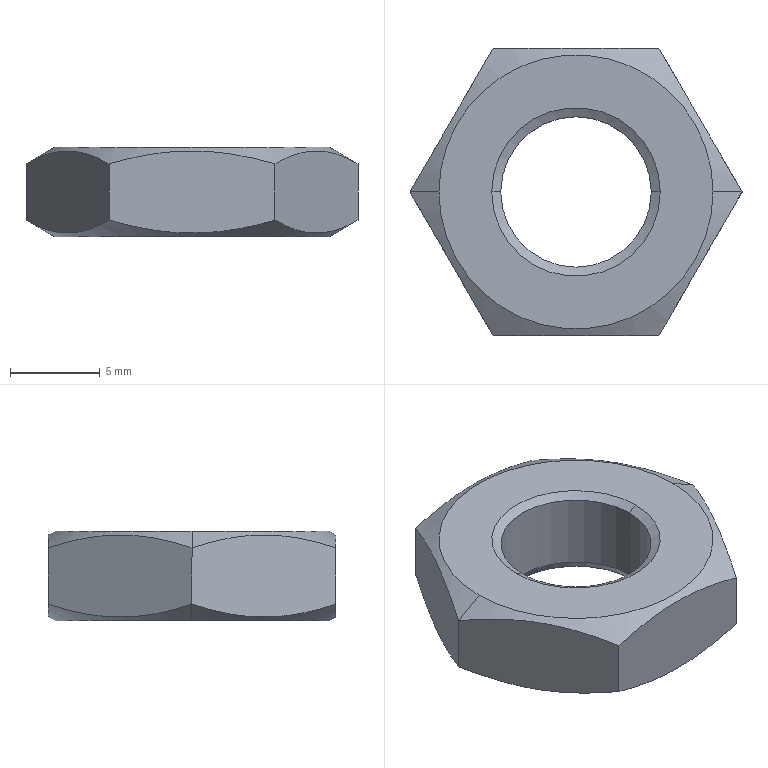Part | SolidWorks | features RevCut 2, Chamfer 1, Extrusion 1, LPattern 1 | 1 solid | 18 faces | box 18.475 x 16 x 5 mm | volume 807.232 mm3 | cone 8 | plane 8 | cylinder 2 | commonest cylinder face diameters 8.376 x2
STEP:
#1=CARTESIAN_POINT('',(-4.188,0.,-0.2887));
#2=VERTEX_POINT('',#1);
#3=CARTESIAN_POINT('',(4.188,0.,-0.2887));
#4=VERTEX_POINT('',#3);
#5=CARTESIAN_POINT('',(0.,0.,-0.2887));
#6=DIRECTION('',(0.,0.,1.));
#7=DIRECTION('',(-1.,0.,0.));
#8=AXIS2_PLACEMENT_3D('',#5,#6,#7);
#9=CIRCLE('',#8,4.188);
#10=EDGE_CURVE('',#2,#4,#9,.T.);
#11=ORIENTED_EDGE('',*,*,#10,.F.);
#12=CARTESIAN_POINT('',(-4.688,0.,0.));
#13=VERTEX_POINT('',#12);
#14=CARTESIAN_POINT('',(-4.188,0.,-0.2887));
#15=DIRECTION('',(-0.866,0.,0.5));
#16=VECTOR('',#15,1000.);
#17=LINE('',#14,#16);
#18=EDGE_CURVE('',#2,#13,#17,.T.);
#19=ORIENTED_EDGE('',*,*,#18,.T.);
#20=CARTESIAN_POINT('',(4.688,0.,0.));
#21=VERTEX_POINT('',#20);
#22=CARTESIAN_POINT('',(0.,0.,0.));
#23=DIRECTION('',(0.,0.,-1.));
#24=DIRECTION('',(-1.,0.,0.));
#25=AXIS2_PLACEMENT_3D('',#22,#23,#24);
#26=CIRCLE('',#25,4.688);
#27=EDGE_CURVE('',#21,#13,#26,.T.);
#28=ORIENTED_EDGE('',*,*,#27,.F.);
#29=CARTESIAN_POINT('',(4.188,0.,-0.2887));
#30=DIRECTION('',(0.866,0.,0.5));
#31=VECTOR('',#30,1000.);
#32=LINE('',#29,#31);
#33=EDGE_CURVE('',#4,#21,#32,.T.);
#34=ORIENTED_EDGE('',*,*,#33,.F.);
#35=EDGE_LOOP('',(#11,#19,#28,#34));
#36=FACE_OUTER_BOUND('',#35,.T.);
#37=CARTESIAN_POINT('',(0.,0.,-0.2887));
#38=DIRECTION('',(0.,0.,1.));
#39=DIRECTION('',(1.,0.,0.));
#40=AXIS2_PLACEMENT_3D('',#37,#38,#39);
#41=CONICAL_SURFACE('',#40,4.188,1.047);
#42=ADVANCED_FACE('',(#36),#41,.F.);
#43=CARTESIAN_POINT('',(4.188,0.,-4.5));
#44=VERTEX_POINT('',#43);
#45=CARTESIAN_POINT('',(-4.188,0.,-4.5));
#46=VERTEX_POINT('',#45);
#47=CARTESIAN_POINT('',(0.,0.,-4.5));
#48=DIRECTION('',(0.,0.,-1.));
#49=DIRECTION('',(-1.,0.,0.));
#50=AXIS2_PLACEMENT_3D('',#47,#48,#49);
#51=CIRCLE('',#50,4.188);
#52=EDGE_CURVE('',#44,#46,#51,.T.);
#53=ORIENTED_EDGE('',*,*,#52,.F.);
#54=CARTESIAN_POINT('',(4.477,0.,-5.));
#55=VERTEX_POINT('',#54);
#56=CARTESIAN_POINT('',(4.477,0.,-5.));
#57=DIRECTION('',(0.5,0.,-0.866));
#58=VECTOR('',#57,1000.);
#59=LINE('',#56,#58);
#60=EDGE_CURVE('',#44,#55,#59,.T.);
#61=ORIENTED_EDGE('',*,*,#60,.T.);
#62=CARTESIAN_POINT('',(-4.477,0.,-5.));
#63=VERTEX_POINT('',#62);
#64=CARTESIAN_POINT('',(0.,0.,-5.));
#65=DIRECTION('',(0.,0.,1.));
#66=DIRECTION('',(-1.,0.,0.));
#67=AXIS2_PLACEMENT_3D('',#64,#65,#66);
#68=CIRCLE('',#67,4.477);
#69=EDGE_CURVE('',#63,#55,#68,.T.);
#70=ORIENTED_EDGE('',*,*,#69,.F.);
#71=CARTESIAN_POINT('',(-4.477,0.,-5.));
#72=DIRECTION('',(-0.5,0.,-0.866));
#73=VECTOR('',#72,1000.);
#74=LINE('',#71,#73);
#75=EDGE_CURVE('',#46,#63,#74,.T.);
#76=ORIENTED_EDGE('',*,*,#75,.F.);
#77=EDGE_LOOP('',(#53,#61,#70,#76));
#78=FACE_OUTER_BOUND('',#77,.T.);
#79=CARTESIAN_POINT('',(0.,0.,-5.));
#80=DIRECTION('',(0.,0.,-1.));
#81=DIRECTION('',(-1.,0.,0.));
#82=AXIS2_PLACEMENT_3D('',#79,#80,#81);
#83=CONICAL_SURFACE('',#82,4.477,0.5236);
#84=ADVANCED_FACE('',(#78),#83,.F.);
#85=CARTESIAN_POINT('',(-7.625,0.,0.));
#86=VERTEX_POINT('',#85);
#87=CARTESIAN_POINT('',(7.625,0.,0.));
#88=VERTEX_POINT('',#87);
#89=CARTESIAN_POINT('',(0.,0.,0.));
#90=DIRECTION('',(0.,0.,-1.));
#91=DIRECTION('',(-1.,0.,0.));
#92=AXIS2_PLACEMENT_3D('',#89,#90,#91);
#93=CIRCLE('',#92,7.625);
#94=EDGE_CURVE('',#86,#88,#93,.T.);
#95=ORIENTED_EDGE('',*,*,#94,.T.);
#96=CARTESIAN_POINT('',(9.238,0.,-0.931));
#97=VERTEX_POINT('',#96);
#98=CARTESIAN_POINT('',(7.625,0.,0.));
#99=DIRECTION('',(0.866,0.,-0.5));
#100=VECTOR('',#99,1000.);
#101=LINE('',#98,#100);
#102=EDGE_CURVE('',#88,#97,#101,.T.);
#103=ORIENTED_EDGE('',*,*,#102,.T.);
#104=CARTESIAN_POINT('',(4.619,8.,-0.931));
#105=VERTEX_POINT('',#104);
#106=CARTESIAN_POINT('',(9.238,0.,-0.931));
#107=CARTESIAN_POINT('',(8.861,0.6531,-0.7133));
#108=CARTESIAN_POINT('',(8.481,1.311,-0.5339));
#109=CARTESIAN_POINT('',(7.713,2.641,-0.2853));
#110=CARTESIAN_POINT('',(7.325,3.312,-0.217));
#111=CARTESIAN_POINT('',(6.736,4.332,-0.2163));
#112=CARTESIAN_POINT('',(6.539,4.674,-0.233));
#113=CARTESIAN_POINT('',(6.149,5.35,-0.2981));
#114=CARTESIAN_POINT('',(5.955,5.686,-0.3464));
#115=CARTESIAN_POINT('',(5.377,6.687,-0.5332));
#116=CARTESIAN_POINT('',(4.996,7.346,-0.7131));
#117=CARTESIAN_POINT('',(4.619,8.,-0.931));
#118=B_SPLINE_CURVE_WITH_KNOTS('',3,(#106,#107,#108,#109,#110,#111,#112,#113,#114,#115,#116,#117),.UNSPECIFIED.,.F.,.F.,(4,2,2,2,2,4),(0.000000238,0.002333,0.004665,0.005831,0.006997,0.00933),.UNSPECIFIED.);
#119=EDGE_CURVE('',#97,#105,#118,.T.);
#120=ORIENTED_EDGE('',*,*,#119,.T.);
#121=CARTESIAN_POINT('',(-4.619,8.,-0.931));
#122=VERTEX_POINT('',#121);
#123=CARTESIAN_POINT('',(4.619,8.,-0.931));
#124=CARTESIAN_POINT('',(3.872,8.,-0.7155));
#125=CARTESIAN_POINT('',(3.116,8.,-0.536));
#126=CARTESIAN_POINT('',(1.573,8.,-0.2855));
#127=CARTESIAN_POINT('',(0.782,8.,-0.2166));
#128=CARTESIAN_POINT('',(-0.7793,8.,-0.2164));
#129=CARTESIAN_POINT('',(-1.555,8.,-0.2835));
#130=CARTESIAN_POINT('',(-3.098,8.,-0.5322));
#131=CARTESIAN_POINT('',(-3.867,8.,-0.7141));
#132=CARTESIAN_POINT('',(-4.619,8.,-0.931));
#133=B_SPLINE_CURVE_WITH_KNOTS('',3,(#123,#124,#125,#126,#127,#128,#129,#130,#131,#132),.UNSPECIFIED.,.F.,.F.,(4,2,2,2,4),(0.003422,0.005753,0.008084,0.01041,0.01275),.UNSPECIFIED.);
#134=EDGE_CURVE('',#105,#122,#133,.T.);
#135=ORIENTED_EDGE('',*,*,#134,.T.);
#136=CARTESIAN_POINT('',(-9.238,0.,-0.931));
#137=VERTEX_POINT('',#136);
#138=CARTESIAN_POINT('',(-4.619,8.,-0.931));
#139=CARTESIAN_POINT('',(-4.996,7.347,-0.7133));
#140=CARTESIAN_POINT('',(-5.376,6.689,-0.5339));
#141=CARTESIAN_POINT('',(-6.143,5.359,-0.2853));
#142=CARTESIAN_POINT('',(-6.531,4.688,-0.217));
#143=CARTESIAN_POINT('',(-7.12,3.668,-0.2163));
#144=CARTESIAN_POINT('',(-7.317,3.326,-0.233));
#145=CARTESIAN_POINT('',(-7.708,2.65,-0.2981));
#146=CARTESIAN_POINT('',(-7.901,2.314,-0.3464));
#147=CARTESIAN_POINT('',(-8.479,1.313,-0.5332));
#148=CARTESIAN_POINT('',(-8.86,0.6539,-0.7131));
#149=CARTESIAN_POINT('',(-9.238,0.,-0.931));
#150=B_SPLINE_CURVE_WITH_KNOTS('',3,(#138,#139,#140,#141,#142,#143,#144,#145,#146,#147,#148,#149),.UNSPECIFIED.,.F.,.F.,(4,2,2,2,2,4),(0.000000238,0.002333,0.004665,0.005831,0.006997,0.00933),.UNSPECIFIED.);
#151=EDGE_CURVE('',#122,#137,#150,.T.);
#152=ORIENTED_EDGE('',*,*,#151,.T.);
#153=CARTESIAN_POINT('',(-7.625,0.,0.));
#154=DIRECTION('',(-0.866,0.,-0.5));
#155=VECTOR('',#154,1000.);
#156=LINE('',#153,#155);
#157=EDGE_CURVE('',#86,#137,#156,.T.);
#158=ORIENTED_EDGE('',*,*,#157,.F.);
#159=EDGE_LOOP('',(#95,#103,#120,#135,#152,#158));
#160=FACE_OUTER_BOUND('',#159,.T.);
#161=CARTESIAN_POINT('',(0.,0.,0.));
#162=DIRECTION('',(0.,0.,-1.));
#163=DIRECTION('',(-1.,0.,0.));
#164=AXIS2_PLACEMENT_3D('',#161,#162,#163);
#165=CONICAL_SURFACE('',#164,7.625,1.047);
#166=ADVANCED_FACE('',(#160),#165,.T.);
#167=CARTESIAN_POINT('',(-7.625,0.,-5.));
#168=VERTEX_POINT('',#167);
#169=CARTESIAN_POINT('',(7.625,0.,-5.));
#170=VERTEX_POINT('',#169);
#171=CARTESIAN_POINT('',(0.,0.,-5.));
#172=DIRECTION('',(0.,0.,-1.));
#173=DIRECTION('',(-1.,0.,0.));
#174=AXIS2_PLACEMENT_3D('',#171,#172,#173);
#175=CIRCLE('',#174,7.625);
#176=EDGE_CURVE('',#168,#170,#175,.T.);
#177=ORIENTED_EDGE('',*,*,#176,.F.);
#178=CARTESIAN_POINT('',(-9.238,0.,-4.069));
#179=VERTEX_POINT('',#178);
#180=CARTESIAN_POINT('',(-9.238,0.,-4.069));
#181=DIRECTION('',(-0.866,0.,0.5));
#182=VECTOR('',#181,1000.);
#183=LINE('',#180,#182);
#184=EDGE_CURVE('',#168,#179,#183,.T.);
#185=ORIENTED_EDGE('',*,*,#184,.T.);
#186=CARTESIAN_POINT('',(-4.619,8.,-4.069));
#187=VERTEX_POINT('',#186);
#188=CARTESIAN_POINT('',(-9.238,0.,-4.069));
#189=CARTESIAN_POINT('',(-8.861,0.6531,-4.287));
#190=CARTESIAN_POINT('',(-8.481,1.311,-4.466));
#191=CARTESIAN_POINT('',(-7.713,2.641,-4.715));
#192=CARTESIAN_POINT('',(-7.325,3.312,-4.783));
#193=CARTESIAN_POINT('',(-6.736,4.332,-4.784));
#194=CARTESIAN_POINT('',(-6.539,4.674,-4.767));
#195=CARTESIAN_POINT('',(-6.149,5.35,-4.702));
#196=CARTESIAN_POINT('',(-5.955,5.686,-4.654));
#197=CARTESIAN_POINT('',(-5.377,6.687,-4.467));
#198=CARTESIAN_POINT('',(-4.996,7.346,-4.287));
#199=CARTESIAN_POINT('',(-4.619,8.,-4.069));
#200=B_SPLINE_CURVE_WITH_KNOTS('',3,(#188,#189,#190,#191,#192,#193,#194,#195,#196,#197,#198,#199),.UNSPECIFIED.,.F.,.F.,(4,2,2,2,2,4),(0.000000238,0.002333,0.004665,0.005831,0.006997,0.00933),.UNSPECIFIED.);
#201=EDGE_CURVE('',#179,#187,#200,.T.);
#202=ORIENTED_EDGE('',*,*,#201,.T.);
#203=CARTESIAN_POINT('',(4.619,8.,-4.069));
#204=VERTEX_POINT('',#203);
#205=CARTESIAN_POINT('',(-4.619,8.,-4.069));
#206=CARTESIAN_POINT('',(-3.867,8.,-4.286));
#207=CARTESIAN_POINT('',(-3.098,8.,-4.468));
#208=CARTESIAN_POINT('',(-1.555,8.,-4.717));
#209=CARTESIAN_POINT('',(-0.7793,8.,-4.784));
#210=CARTESIAN_POINT('',(0.782,8.,-4.783));
#211=CARTESIAN_POINT('',(1.573,8.,-4.714));
#212=CARTESIAN_POINT('',(3.116,8.,-4.464));
#213=CARTESIAN_POINT('',(3.872,8.,-4.284));
#214=CARTESIAN_POINT('',(4.619,8.,-4.069));
#215=B_SPLINE_CURVE_WITH_KNOTS('',3,(#205,#206,#207,#208,#209,#210,#211,#212,#213,#214),.UNSPECIFIED.,.F.,.F.,(4,2,2,2,4),(0.008207,0.01054,0.01288,0.01522,0.01755),.UNSPECIFIED.);
#216=EDGE_CURVE('',#187,#204,#215,.T.);
#217=ORIENTED_EDGE('',*,*,#216,.T.);
#218=CARTESIAN_POINT('',(9.238,0.,-4.069));
#219=VERTEX_POINT('',#218);
#220=CARTESIAN_POINT('',(4.619,8.,-4.069));
#221=CARTESIAN_POINT('',(4.996,7.347,-4.287));
#222=CARTESIAN_POINT('',(5.376,6.689,-4.466));
#223=CARTESIAN_POINT('',(6.143,5.359,-4.715));
#224=CARTESIAN_POINT('',(6.531,4.688,-4.783));
#225=CARTESIAN_POINT('',(7.12,3.668,-4.784));
#226=CARTESIAN_POINT('',(7.317,3.326,-4.767));
#227=CARTESIAN_POINT('',(7.708,2.65,-4.702));
#228=CARTESIAN_POINT('',(7.901,2.314,-4.654));
#229=CARTESIAN_POINT('',(8.479,1.313,-4.467));
#230=CARTESIAN_POINT('',(8.86,0.6539,-4.287));
#231=CARTESIAN_POINT('',(9.238,0.,-4.069));
#232=B_SPLINE_CURVE_WITH_KNOTS('',3,(#220,#221,#222,#223,#224,#225,#226,#227,#228,#229,#230,#231),.UNSPECIFIED.,.F.,.F.,(4,2,2,2,2,4),(0.000000238,0.002333,0.004665,0.005831,0.006997,0.00933),.UNSPECIFIED.);
#233=EDGE_CURVE('',#204,#219,#232,.T.);
#234=ORIENTED_EDGE('',*,*,#233,.T.);
#235=CARTESIAN_POINT('',(9.238,0.,-4.069));
#236=DIRECTION('',(0.866,0.,0.5));
#237=VECTOR('',#236,1000.);
#238=LINE('',#235,#237);
#239=EDGE_CURVE('',#170,#219,#238,.T.);
#240=ORIENTED_EDGE('',*,*,#239,.F.);
#241=EDGE_LOOP('',(#177,#185,#202,#217,#234,#240));
#242=FACE_OUTER_BOUND('',#241,.T.);
#243=CARTESIAN_POINT('',(0.,0.,-4.069));
#244=DIRECTION('',(0.,0.,1.));
#245=DIRECTION('',(1.,0.,0.));
#246=AXIS2_PLACEMENT_3D('',#243,#244,#245);
#247=CONICAL_SURFACE('',#246,9.238,1.047);
#248=ADVANCED_FACE('',(#242),#247,.T.);
#249=ORIENTED_EDGE('',*,*,#52,.T.);
#250=CARTESIAN_POINT('',(-4.188,0.,-5.));
#251=DIRECTION('',(0.,0.,1.));
#252=VECTOR('',#251,1000.);
#253=LINE('',#250,#252);
#254=EDGE_CURVE('',#46,#2,#253,.T.);
#255=ORIENTED_EDGE('',*,*,#254,.T.);
#256=ORIENTED_EDGE('',*,*,#10,.T.);
#257=CARTESIAN_POINT('',(4.188,0.,-5.));
#258=DIRECTION('',(0.,0.,1.));
#259=VECTOR('',#258,1000.);
#260=LINE('',#257,#259);
#261=EDGE_CURVE('',#44,#4,#260,.T.);
#262=ORIENTED_EDGE('',*,*,#261,.F.);
#263=EDGE_LOOP('',(#249,#255,#256,#262));
#264=FACE_OUTER_BOUND('',#263,.T.);
#265=CARTESIAN_POINT('',(0.,0.,-5.));
#266=DIRECTION('',(0.,0.,1.));
#267=DIRECTION('',(1.,0.,0.));
#268=AXIS2_PLACEMENT_3D('',#265,#266,#267);
#269=CYLINDRICAL_SURFACE('',#268,4.188);
#270=ADVANCED_FACE('',(#264),#269,.F.);
#271=CARTESIAN_POINT('',(-4.619,-8.,-0.931));
#272=VERTEX_POINT('',#271);
#273=CARTESIAN_POINT('',(4.619,-8.,-0.931));
#274=VERTEX_POINT('',#273);
#275=CARTESIAN_POINT('',(-4.619,-8.,-0.931));
#276=CARTESIAN_POINT('',(-3.867,-8.,-0.7141));
#277=CARTESIAN_POINT('',(-3.098,-8.,-0.5322));
#278=CARTESIAN_POINT('',(-1.555,-8.,-0.2835));
#279=CARTESIAN_POINT('',(-0.7793,-8.,-0.2164));
#280=CARTESIAN_POINT('',(0.782,-8.,-0.2166));
#281=CARTESIAN_POINT('',(1.573,-8.,-0.2855));
#282=CARTESIAN_POINT('',(3.116,-8.,-0.536));
#283=CARTESIAN_POINT('',(3.872,-8.,-0.7155));
#284=CARTESIAN_POINT('',(4.619,-8.,-0.931));
#285=B_SPLINE_CURVE_WITH_KNOTS('',3,(#275,#276,#277,#278,#279,#280,#281,#282,#283,#284),.UNSPECIFIED.,.F.,.F.,(4,2,2,2,4),(0.008207,0.01054,0.01288,0.01522,0.01755),.UNSPECIFIED.);
#286=EDGE_CURVE('',#272,#274,#285,.T.);
#287=ORIENTED_EDGE('',*,*,#286,.F.);
#288=CARTESIAN_POINT('',(-4.619,-8.,-4.069));
#289=VERTEX_POINT('',#288);
#290=CARTESIAN_POINT('',(-4.619,-8.,-5.));
#291=DIRECTION('',(0.,0.,1.));
#292=VECTOR('',#291,1000.);
#293=LINE('',#290,#292);
#294=EDGE_CURVE('',#289,#272,#293,.T.);
#295=ORIENTED_EDGE('',*,*,#294,.F.);
#296=CARTESIAN_POINT('',(4.619,-8.,-4.069));
#297=VERTEX_POINT('',#296);
#298=CARTESIAN_POINT('',(4.619,-8.,-4.069));
#299=CARTESIAN_POINT('',(3.872,-8.,-4.284));
#300=CARTESIAN_POINT('',(3.116,-8.,-4.464));
#301=CARTESIAN_POINT('',(1.573,-8.,-4.714));
#302=CARTESIAN_POINT('',(0.782,-8.,-4.783));
#303=CARTESIAN_POINT('',(-0.7793,-8.,-4.784));
#304=CARTESIAN_POINT('',(-1.555,-8.,-4.717));
#305=CARTESIAN_POINT('',(-3.098,-8.,-4.468));
#306=CARTESIAN_POINT('',(-3.867,-8.,-4.286));
#307=CARTESIAN_POINT('',(-4.619,-8.,-4.069));
#308=B_SPLINE_CURVE_WITH_KNOTS('',3,(#298,#299,#300,#301,#302,#303,#304,#305,#306,#307),.UNSPECIFIED.,.F.,.F.,(4,2,2,2,4),(0.003422,0.005753,0.008084,0.01041,0.01275),.UNSPECIFIED.);
#309=EDGE_CURVE('',#297,#289,#308,.T.);
#310=ORIENTED_EDGE('',*,*,#309,.F.);
#311=CARTESIAN_POINT('',(4.619,-8.,-5.));
#312=DIRECTION('',(0.,0.,1.));
#313=VECTOR('',#312,1000.);
#314=LINE('',#311,#313);
#315=EDGE_CURVE('',#297,#274,#314,.T.);
#316=ORIENTED_EDGE('',*,*,#315,.T.);
#317=EDGE_LOOP('',(#287,#295,#310,#316));
#318=FACE_OUTER_BOUND('',#317,.T.);
#319=CARTESIAN_POINT('',(-4.619,-8.,-5.));
#320=DIRECTION('',(0.,-1.,0.));
#321=DIRECTION('',(1.,0.,0.));
#322=AXIS2_PLACEMENT_3D('',#319,#320,#321);
#323=PLANE('',#322);
#324=ADVANCED_FACE('',(#318),#323,.T.);
#325=CARTESIAN_POINT('',(-9.238,0.,-0.931));
#326=CARTESIAN_POINT('',(-8.861,-0.6531,-0.7133));
#327=CARTESIAN_POINT('',(-8.481,-1.311,-0.5339));
#328=CARTESIAN_POINT('',(-7.713,-2.641,-0.2853));
#329=CARTESIAN_POINT('',(-7.325,-3.312,-0.217));
#330=CARTESIAN_POINT('',(-6.736,-4.332,-0.2163));
#331=CARTESIAN_POINT('',(-6.539,-4.674,-0.233));
#332=CARTESIAN_POINT('',(-6.149,-5.35,-0.2981));
#333=CARTESIAN_POINT('',(-5.955,-5.686,-0.3464));
#334=CARTESIAN_POINT('',(-5.377,-6.687,-0.5332));
#335=CARTESIAN_POINT('',(-4.996,-7.346,-0.7131));
#336=CARTESIAN_POINT('',(-4.619,-8.,-0.931));
#337=B_SPLINE_CURVE_WITH_KNOTS('',3,(#325,#326,#327,#328,#329,#330,#331,#332,#333,#334,#335,#336),.UNSPECIFIED.,.F.,.F.,(4,2,2,2,2,4),(0.000000238,0.002333,0.004665,0.005831,0.006997,0.00933),.UNSPECIFIED.);
#338=EDGE_CURVE('',#137,#272,#337,.T.);
#339=ORIENTED_EDGE('',*,*,#338,.F.);
#340=CARTESIAN_POINT('',(-9.238,0.,-5.));
#341=DIRECTION('',(0.,0.,1.));
#342=VECTOR('',#341,1000.);
#343=LINE('',#340,#342);
#344=EDGE_CURVE('',#179,#137,#343,.T.);
#345=ORIENTED_EDGE('',*,*,#344,.F.);
#346=CARTESIAN_POINT('',(-4.619,-8.,-4.069));
#347=CARTESIAN_POINT('',(-4.996,-7.347,-4.287));
#348=CARTESIAN_POINT('',(-5.376,-6.689,-4.466));
#349=CARTESIAN_POINT('',(-6.143,-5.359,-4.715));
#350=CARTESIAN_POINT('',(-6.531,-4.688,-4.783));
#351=CARTESIAN_POINT('',(-7.12,-3.668,-4.784));
#352=CARTESIAN_POINT('',(-7.317,-3.326,-4.767));
#353=CARTESIAN_POINT('',(-7.708,-2.65,-4.702));
#354=CARTESIAN_POINT('',(-7.901,-2.314,-4.654));
#355=CARTESIAN_POINT('',(-8.479,-1.313,-4.467));
#356=CARTESIAN_POINT('',(-8.86,-0.6539,-4.287));
#357=CARTESIAN_POINT('',(-9.238,0.,-4.069));
#358=B_SPLINE_CURVE_WITH_KNOTS('',3,(#346,#347,#348,#349,#350,#351,#352,#353,#354,#355,#356,#357),.UNSPECIFIED.,.F.,.F.,(4,2,2,2,2,4),(0.000000238,0.002333,0.004665,0.005831,0.006997,0.00933),.UNSPECIFIED.);
#359=EDGE_CURVE('',#289,#179,#358,.T.);
#360=ORIENTED_EDGE('',*,*,#359,.F.);
#361=ORIENTED_EDGE('',*,*,#294,.T.);
#362=EDGE_LOOP('',(#339,#345,#360,#361));
#363=FACE_OUTER_BOUND('',#362,.T.);
#364=CARTESIAN_POINT('',(-9.238,0.,-5.));
#365=DIRECTION('',(-0.866,-0.5,0.));
#366=DIRECTION('',(0.5,-0.866,0.));
#367=AXIS2_PLACEMENT_3D('',#364,#365,#366);
#368=PLANE('',#367);
#369=ADVANCED_FACE('',(#363),#368,.T.);
#370=ORIENTED_EDGE('',*,*,#151,.F.);
#371=CARTESIAN_POINT('',(-4.619,8.,-5.));
#372=DIRECTION('',(0.,0.,1.));
#373=VECTOR('',#372,1000.);
#374=LINE('',#371,#373);
#375=EDGE_CURVE('',#187,#122,#374,.T.);
#376=ORIENTED_EDGE('',*,*,#375,.F.);
#377=ORIENTED_EDGE('',*,*,#201,.F.);
#378=ORIENTED_EDGE('',*,*,#344,.T.);
#379=EDGE_LOOP('',(#370,#376,#377,#378));
#380=FACE_OUTER_BOUND('',#379,.T.);
#381=CARTESIAN_POINT('',(-4.619,8.,-5.));
#382=DIRECTION('',(-0.866,0.5,0.));
#383=DIRECTION('',(-0.5,-0.866,0.));
#384=AXIS2_PLACEMENT_3D('',#381,#382,#383);
#385=PLANE('',#384);
#386=ADVANCED_FACE('',(#380),#385,.T.);
#387=ORIENTED_EDGE('',*,*,#134,.F.);
#388=CARTESIAN_POINT('',(4.619,8.,-5.));
#389=DIRECTION('',(0.,0.,1.));
#390=VECTOR('',#389,1000.);
#391=LINE('',#388,#390);
#392=EDGE_CURVE('',#204,#105,#391,.T.);
#393=ORIENTED_EDGE('',*,*,#392,.F.);
#394=ORIENTED_EDGE('',*,*,#216,.F.);
#395=ORIENTED_EDGE('',*,*,#375,.T.);
#396=EDGE_LOOP('',(#387,#393,#394,#395));
#397=FACE_OUTER_BOUND('',#396,.T.);
#398=CARTESIAN_POINT('',(4.619,8.,-5.));
#399=DIRECTION('',(0.,1.,0.));
#400=DIRECTION('',(0.,0.,1.));
#401=AXIS2_PLACEMENT_3D('',#398,#399,#400);
#402=PLANE('',#401);
#403=ADVANCED_FACE('',(#397),#402,.T.);
#404=ORIENTED_EDGE('',*,*,#119,.F.);
#405=CARTESIAN_POINT('',(9.238,0.,-5.));
#406=DIRECTION('',(0.,0.,1.));
#407=VECTOR('',#406,1000.);
#408=LINE('',#405,#407);
#409=EDGE_CURVE('',#219,#97,#408,.T.);
#410=ORIENTED_EDGE('',*,*,#409,.F.);
#411=ORIENTED_EDGE('',*,*,#233,.F.);
#412=ORIENTED_EDGE('',*,*,#392,.T.);
#413=EDGE_LOOP('',(#404,#410,#411,#412));
#414=FACE_OUTER_BOUND('',#413,.T.);
#415=CARTESIAN_POINT('',(9.238,0.,-5.));
#416=DIRECTION('',(0.866,0.5,0.));
#417=DIRECTION('',(-0.5,0.866,0.));
#418=AXIS2_PLACEMENT_3D('',#415,#416,#417);
#419=PLANE('',#418);
#420=ADVANCED_FACE('',(#414),#419,.T.);
#421=CARTESIAN_POINT('',(4.619,-8.,-0.931));
#422=CARTESIAN_POINT('',(4.996,-7.347,-0.7133));
#423=CARTESIAN_POINT('',(5.376,-6.689,-0.5339));
#424=CARTESIAN_POINT('',(6.143,-5.359,-0.2853));
#425=CARTESIAN_POINT('',(6.531,-4.688,-0.217));
#426=CARTESIAN_POINT('',(7.12,-3.668,-0.2163));
#427=CARTESIAN_POINT('',(7.317,-3.326,-0.233));
#428=CARTESIAN_POINT('',(7.708,-2.65,-0.2981));
#429=CARTESIAN_POINT('',(7.901,-2.314,-0.3464));
#430=CARTESIAN_POINT('',(8.479,-1.313,-0.5332));
#431=CARTESIAN_POINT('',(8.86,-0.6539,-0.7131));
#432=CARTESIAN_POINT('',(9.238,0.,-0.931));
#433=B_SPLINE_CURVE_WITH_KNOTS('',3,(#421,#422,#423,#424,#425,#426,#427,#428,#429,#430,#431,#432),.UNSPECIFIED.,.F.,.F.,(4,2,2,2,2,4),(0.000000238,0.002333,0.004665,0.005831,0.006997,0.00933),.UNSPECIFIED.);
#434=EDGE_CURVE('',#274,#97,#433,.T.);
#435=ORIENTED_EDGE('',*,*,#434,.F.);
#436=ORIENTED_EDGE('',*,*,#315,.F.);
#437=CARTESIAN_POINT('',(9.238,0.,-4.069));
#438=CARTESIAN_POINT('',(8.861,-0.6531,-4.287));
#439=CARTESIAN_POINT('',(8.481,-1.311,-4.466));
#440=CARTESIAN_POINT('',(7.713,-2.641,-4.715));
#441=CARTESIAN_POINT('',(7.325,-3.312,-4.783));
#442=CARTESIAN_POINT('',(6.736,-4.332,-4.784));
#443=CARTESIAN_POINT('',(6.539,-4.674,-4.767));
#444=CARTESIAN_POINT('',(6.149,-5.35,-4.702));
#445=CARTESIAN_POINT('',(5.955,-5.686,-4.654));
#446=CARTESIAN_POINT('',(5.377,-6.687,-4.467));
#447=CARTESIAN_POINT('',(4.996,-7.346,-4.287));
#448=CARTESIAN_POINT('',(4.619,-8.,-4.069));
#449=B_SPLINE_CURVE_WITH_KNOTS('',3,(#437,#438,#439,#440,#441,#442,#443,#444,#445,#446,#447,#448),.UNSPECIFIED.,.F.,.F.,(4,2,2,2,2,4),(0.000000238,0.002333,0.004665,0.005831,0.006997,0.00933),.UNSPECIFIED.);
#450=EDGE_CURVE('',#219,#297,#449,.T.);
#451=ORIENTED_EDGE('',*,*,#450,.F.);
#452=ORIENTED_EDGE('',*,*,#409,.T.);
#453=EDGE_LOOP('',(#435,#436,#451,#452));
#454=FACE_OUTER_BOUND('',#453,.T.);
#455=CARTESIAN_POINT('',(4.619,-8.,-5.));
#456=DIRECTION('',(0.866,-0.5,0.));
#457=DIRECTION('',(0.5,0.866,0.));
#458=AXIS2_PLACEMENT_3D('',#455,#456,#457);
#459=PLANE('',#458);
#460=ADVANCED_FACE('',(#454),#459,.T.);
#461=ORIENTED_EDGE('',*,*,#69,.T.);
#462=CARTESIAN_POINT('',(0.,0.,-5.));
#463=DIRECTION('',(0.,0.,1.));
#464=DIRECTION('',(-1.,0.,0.));
#465=AXIS2_PLACEMENT_3D('',#462,#463,#464);
#466=CIRCLE('',#465,4.477);
#467=EDGE_CURVE('',#55,#63,#466,.T.);
#468=ORIENTED_EDGE('',*,*,#467,.T.);
#469=EDGE_LOOP('',(#461,#468));
#470=FACE_BOUND('',#469,.T.);
#471=CARTESIAN_POINT('',(0.,0.,-5.));
#472=DIRECTION('',(0.,0.,-1.));
#473=DIRECTION('',(-1.,0.,0.));
#474=AXIS2_PLACEMENT_3D('',#471,#472,#473);
#475=CIRCLE('',#474,7.625);
#476=EDGE_CURVE('',#170,#168,#475,.T.);
#477=ORIENTED_EDGE('',*,*,#476,.T.);
#478=ORIENTED_EDGE('',*,*,#176,.T.);
#479=EDGE_LOOP('',(#477,#478));
#480=FACE_OUTER_BOUND('',#479,.T.);
#481=CARTESIAN_POINT('',(-4.619,-8.,-5.));
#482=DIRECTION('',(0.,0.,-1.));
#483=DIRECTION('',(-1.,0.,0.));
#484=AXIS2_PLACEMENT_3D('',#481,#482,#483);
#485=PLANE('',#484);
#486=ADVANCED_FACE('',(#470,#480),#485,.T.);
#487=ORIENTED_EDGE('',*,*,#27,.T.);
#488=CARTESIAN_POINT('',(0.,0.,0.));
#489=DIRECTION('',(0.,0.,-1.));
#490=DIRECTION('',(-1.,0.,0.));
#491=AXIS2_PLACEMENT_3D('',#488,#489,#490);
#492=CIRCLE('',#491,4.688);
#493=EDGE_CURVE('',#13,#21,#492,.T.);
#494=ORIENTED_EDGE('',*,*,#493,.T.);
#495=EDGE_LOOP('',(#487,#494));
#496=FACE_BOUND('',#495,.T.);
#497=ORIENTED_EDGE('',*,*,#94,.F.);
#498=CARTESIAN_POINT('',(0.,0.,0.));
#499=DIRECTION('',(0.,0.,-1.));
#500=DIRECTION('',(-1.,0.,0.));
#501=AXIS2_PLACEMENT_3D('',#498,#499,#500);
#502=CIRCLE('',#501,7.625);
#503=EDGE_CURVE('',#88,#86,#502,.T.);
#504=ORIENTED_EDGE('',*,*,#503,.F.);
#505=EDGE_LOOP('',(#497,#504));
#506=FACE_OUTER_BOUND('',#505,.T.);
#507=CARTESIAN_POINT('',(-4.619,-8.,0.));
#508=DIRECTION('',(0.,0.,-1.));
#509=DIRECTION('',(-1.,0.,0.));
#510=AXIS2_PLACEMENT_3D('',#507,#508,#509);
#511=PLANE('',#510);
#512=ADVANCED_FACE('',(#496,#506),#511,.F.);
#513=ORIENTED_EDGE('',*,*,#254,.F.);
#514=CARTESIAN_POINT('',(0.,0.,-4.5));
#515=DIRECTION('',(0.,0.,-1.));
#516=DIRECTION('',(-1.,0.,0.));
#517=AXIS2_PLACEMENT_3D('',#514,#515,#516);
#518=CIRCLE('',#517,4.188);
#519=EDGE_CURVE('',#46,#44,#518,.T.);
#520=ORIENTED_EDGE('',*,*,#519,.T.);
#521=ORIENTED_EDGE('',*,*,#261,.T.);
#522=CARTESIAN_POINT('',(0.,0.,-0.2887));
#523=DIRECTION('',(0.,0.,1.));
#524=DIRECTION('',(-1.,0.,0.));
#525=AXIS2_PLACEMENT_3D('',#522,#523,#524);
#526=CIRCLE('',#525,4.188);
#527=EDGE_CURVE('',#4,#2,#526,.T.);
#528=ORIENTED_EDGE('',*,*,#527,.T.);
#529=EDGE_LOOP('',(#513,#520,#521,#528));
#530=FACE_OUTER_BOUND('',#529,.T.);
#531=CARTESIAN_POINT('',(0.,0.,-5.));
#532=DIRECTION('',(0.,0.,1.));
#533=DIRECTION('',(1.,0.,0.));
#534=AXIS2_PLACEMENT_3D('',#531,#532,#533);
#535=CYLINDRICAL_SURFACE('',#534,4.188);
#536=ADVANCED_FACE('',(#530),#535,.F.);
#537=ORIENTED_EDGE('',*,*,#184,.F.);
#538=ORIENTED_EDGE('',*,*,#476,.F.);
#539=ORIENTED_EDGE('',*,*,#239,.T.);
#540=ORIENTED_EDGE('',*,*,#450,.T.);
#541=ORIENTED_EDGE('',*,*,#309,.T.);
#542=ORIENTED_EDGE('',*,*,#359,.T.);
#543=EDGE_LOOP('',(#537,#538,#539,#540,#541,#542));
#544=FACE_OUTER_BOUND('',#543,.T.);
#545=CARTESIAN_POINT('',(0.,0.,-4.069));
#546=DIRECTION('',(0.,0.,1.));
#547=DIRECTION('',(1.,0.,0.));
#548=AXIS2_PLACEMENT_3D('',#545,#546,#547);
#549=CONICAL_SURFACE('',#548,9.238,1.047);
#550=ADVANCED_FACE('',(#544),#549,.T.);
#551=ORIENTED_EDGE('',*,*,#102,.F.);
#552=ORIENTED_EDGE('',*,*,#503,.T.);
#553=ORIENTED_EDGE('',*,*,#157,.T.);
#554=ORIENTED_EDGE('',*,*,#338,.T.);
#555=ORIENTED_EDGE('',*,*,#286,.T.);
#556=ORIENTED_EDGE('',*,*,#434,.T.);
#557=EDGE_LOOP('',(#551,#552,#553,#554,#555,#556));
#558=FACE_OUTER_BOUND('',#557,.T.);
#559=CARTESIAN_POINT('',(0.,0.,0.));
#560=DIRECTION('',(0.,0.,-1.));
#561=DIRECTION('',(-1.,0.,0.));
#562=AXIS2_PLACEMENT_3D('',#559,#560,#561);
#563=CONICAL_SURFACE('',#562,7.625,1.047);
#564=ADVANCED_FACE('',(#558),#563,.T.);
#565=ORIENTED_EDGE('',*,*,#60,.F.);
#566=ORIENTED_EDGE('',*,*,#519,.F.);
#567=ORIENTED_EDGE('',*,*,#75,.T.);
#568=ORIENTED_EDGE('',*,*,#467,.F.);
#569=EDGE_LOOP('',(#565,#566,#567,#568));
#570=FACE_OUTER_BOUND('',#569,.T.);
#571=CARTESIAN_POINT('',(0.,0.,-5.));
#572=DIRECTION('',(0.,0.,-1.));
#573=DIRECTION('',(-1.,0.,0.));
#574=AXIS2_PLACEMENT_3D('',#571,#572,#573);
#575=CONICAL_SURFACE('',#574,4.477,0.5236);
#576=ADVANCED_FACE('',(#570),#575,.F.);
#577=ORIENTED_EDGE('',*,*,#18,.F.);
#578=ORIENTED_EDGE('',*,*,#527,.F.);
#579=ORIENTED_EDGE('',*,*,#33,.T.);
#580=ORIENTED_EDGE('',*,*,#493,.F.);
#581=EDGE_LOOP('',(#577,#578,#579,#580));
#582=FACE_OUTER_BOUND('',#581,.T.);
#583=CARTESIAN_POINT('',(0.,0.,-0.2887));
#584=DIRECTION('',(0.,0.,1.));
#585=DIRECTION('',(1.,0.,0.));
#586=AXIS2_PLACEMENT_3D('',#583,#584,#585);
#587=CONICAL_SURFACE('',#586,4.188,1.047);
#588=ADVANCED_FACE('',(#582),#587,.F.);
#589=CLOSED_SHELL('',(#42,#84,#166,#248,#270,#324,#369,#386,#403,#420,#460,#486,#512,#536,#550,#564,#576,#588));
#590=MANIFOLD_SOLID_BREP('',#589);
#591=CARTESIAN_POINT('',(0.,0.,0.));
#592=DIRECTION('',(0.,0.,1.));
#593=DIRECTION('',(1.,0.,0.));
#594=AXIS2_PLACEMENT_3D('',#591,#592,#593);
#595=(LENGTH_UNIT()NAMED_UNIT(*)SI_UNIT(.MILLI.,.METRE.));
#596=UNCERTAINTY_MEASURE_WITH_UNIT(LENGTH_MEASURE(0.00001),#595,'','');
#597=(NAMED_UNIT(*)PLANE_ANGLE_UNIT()SI_UNIT($,.RADIAN.));
#598=(NAMED_UNIT(*)SI_UNIT($,.STERADIAN.)SOLID_ANGLE_UNIT());
#599=(GEOMETRIC_REPRESENTATION_CONTEXT(3)GLOBAL_UNCERTAINTY_ASSIGNED_CONTEXT((#596))GLOBAL_UNIT_ASSIGNED_CONTEXT((#595,#597,#598))REPRESENTATION_CONTEXT('',''));
#600=ADVANCED_BREP_SHAPE_REPRESENTATION('',(#590,#594),#599);